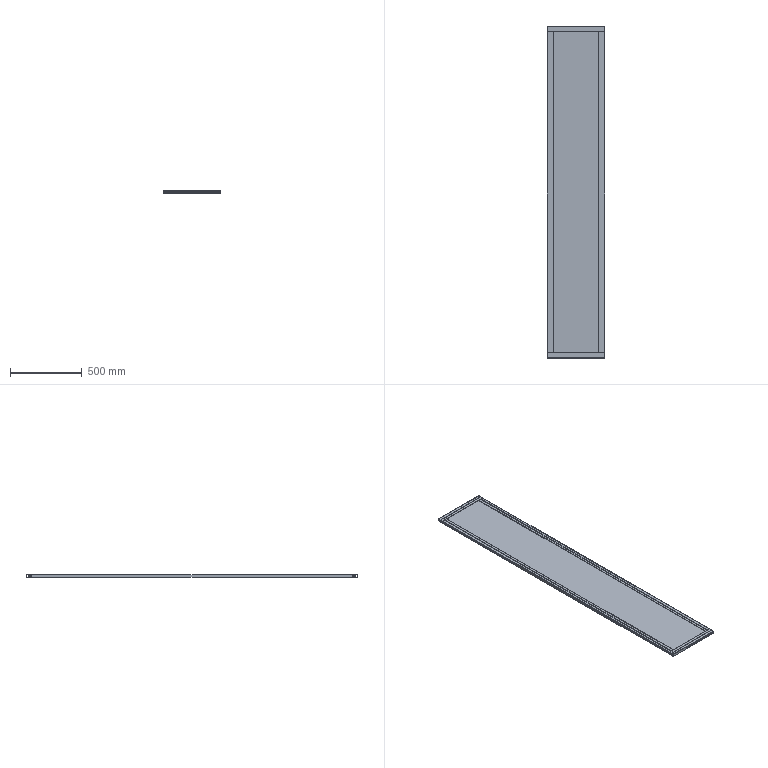Part | SolidWorks | features ICE 1, WeldMemberFeat 1, WeldmentFeature 1 | 5 solids | 158 faces | box 398.5 x 2317 x 18 mm | volume 9317148 mm3 | plane 94 | cylinder 64 | commonest cylinder face diameters 1.1 x24 3.6 x20 5.8 x20